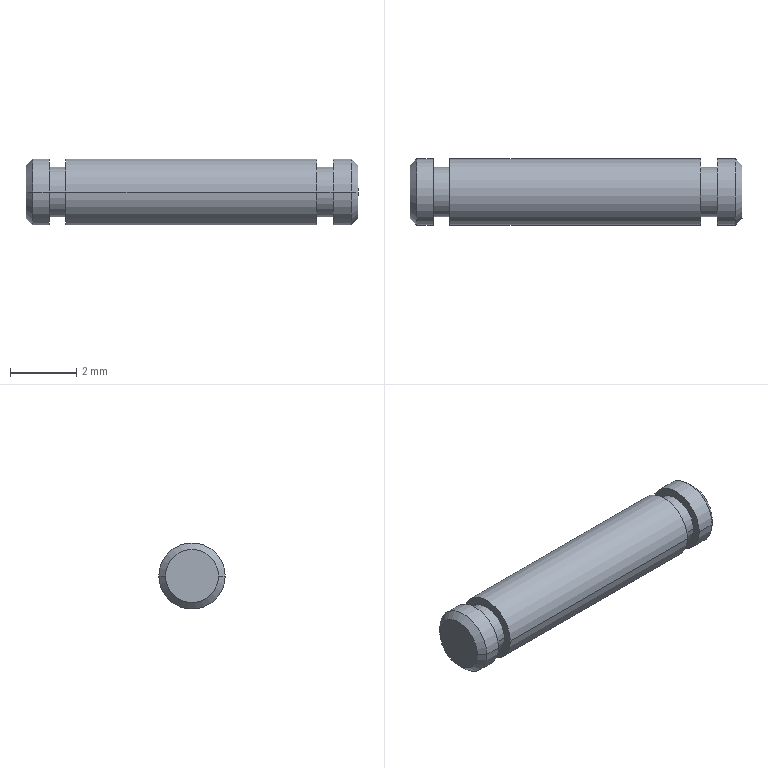Part | NX | 1 solid | 20 faces | box 10 x 2 x 2 mm | volume 29.807 mm3 | cylinder 10 | plane 6 | cone 4 | commonest cylinder face diameters 2 x6 1.5 x4
STEP:
#1=CARTESIAN_POINT('',(-1.16,-50.479,1.703));
#2=VERTEX_POINT('',#1);
#3=CARTESIAN_POINT('',(-1.16,-52.479,1.703));
#4=VERTEX_POINT('',#3);
#5=CARTESIAN_POINT('',(-1.16,-51.479,1.703));
#6=DIRECTION('',(-1.,0.,0.));
#7=DIRECTION('',(0.,-1.,0.));
#8=AXIS2_PLACEMENT_3D('',#5,#6,#7);
#9=CIRCLE('',#8,1.);
#10=EDGE_CURVE('',#2,#4,#9,.T.);
#11=ORIENTED_EDGE('',*,*,#10,.T.);
#12=CARTESIAN_POINT('',(-1.71,-52.479,1.703));
#13=VERTEX_POINT('',#12);
#14=CARTESIAN_POINT('',(-10.96,-52.479,1.703));
#15=DIRECTION('',(-1.,0.,0.));
#16=VECTOR('',#15,1000.);
#17=LINE('',#14,#16);
#18=EDGE_CURVE('',#13,#4,#17,.F.);
#19=ORIENTED_EDGE('',*,*,#18,.F.);
#20=CARTESIAN_POINT('',(-1.71,-50.479,1.703));
#21=VERTEX_POINT('',#20);
#22=CARTESIAN_POINT('',(-1.71,-51.479,1.703));
#23=DIRECTION('',(-1.,0.,0.));
#24=DIRECTION('',(0.,-1.,0.));
#25=AXIS2_PLACEMENT_3D('',#22,#23,#24);
#26=CIRCLE('',#25,1.);
#27=EDGE_CURVE('',#21,#13,#26,.T.);
#28=ORIENTED_EDGE('',*,*,#27,.F.);
#29=CARTESIAN_POINT('',(-10.96,-50.479,1.703));
#30=DIRECTION('',(-1.,0.,0.));
#31=VECTOR('',#30,1000.);
#32=LINE('',#29,#31);
#33=EDGE_CURVE('',#21,#2,#32,.F.);
#34=ORIENTED_EDGE('',*,*,#33,.T.);
#35=EDGE_LOOP('',(#11,#19,#28,#34));
#36=FACE_BOUND('',#35,.T.);
#37=CARTESIAN_POINT('',(-10.96,-51.479,1.703));
#38=DIRECTION('',(-1.,0.,0.));
#39=DIRECTION('',(0.,-1.,0.));
#40=AXIS2_PLACEMENT_3D('',#37,#38,#39);
#41=CYLINDRICAL_SURFACE('',#40,1.);
#42=ADVANCED_FACE('',(#36),#41,.T.);
#43=ORIENTED_EDGE('',*,*,#27,.T.);
#44=CARTESIAN_POINT('',(-1.71,-51.479,1.703));
#45=DIRECTION('',(-1.,0.,0.));
#46=DIRECTION('',(0.,-1.,0.));
#47=AXIS2_PLACEMENT_3D('',#44,#45,#46);
#48=CIRCLE('',#47,1.);
#49=EDGE_CURVE('',#13,#21,#48,.T.);
#50=ORIENTED_EDGE('',*,*,#49,.T.);
#51=EDGE_LOOP('',(#43,#50));
#52=FACE_BOUND('',#51,.T.);
#53=CARTESIAN_POINT('',(-1.71,-50.729,1.703));
#54=VERTEX_POINT('',#53);
#55=CARTESIAN_POINT('',(-1.71,-52.229,1.703));
#56=VERTEX_POINT('',#55);
#57=CARTESIAN_POINT('',(-1.71,-51.479,1.703));
#58=DIRECTION('',(-1.,0.,0.));
#59=DIRECTION('',(0.,-1.,0.));
#60=AXIS2_PLACEMENT_3D('',#57,#58,#59);
#61=CIRCLE('',#60,0.75);
#62=EDGE_CURVE('',#54,#56,#61,.T.);
#63=ORIENTED_EDGE('',*,*,#62,.F.);
#64=CARTESIAN_POINT('',(-1.71,-51.479,1.703));
#65=DIRECTION('',(-1.,0.,0.));
#66=DIRECTION('',(0.,-1.,0.));
#67=AXIS2_PLACEMENT_3D('',#64,#65,#66);
#68=CIRCLE('',#67,0.75);
#69=EDGE_CURVE('',#56,#54,#68,.T.);
#70=ORIENTED_EDGE('',*,*,#69,.F.);
#71=EDGE_LOOP('',(#63,#70));
#72=FACE_BOUND('',#71,.T.);
#73=CARTESIAN_POINT('',(-1.71,-50.265,1.703));
#74=DIRECTION('',(-1.,0.,0.));
#75=DIRECTION('',(0.,1.,0.));
#76=AXIS2_PLACEMENT_3D('',#73,#74,#75);
#77=PLANE('',#76);
#78=ADVANCED_FACE('',(#52,#72),#77,.T.);
#79=CARTESIAN_POINT('',(-2.21,-50.729,1.703));
#80=VERTEX_POINT('',#79);
#81=CARTESIAN_POINT('',(-2.21,-52.229,1.703));
#82=VERTEX_POINT('',#81);
#83=CARTESIAN_POINT('',(-2.21,-51.479,1.703));
#84=DIRECTION('',(-1.,0.,0.));
#85=DIRECTION('',(0.,-1.,0.));
#86=AXIS2_PLACEMENT_3D('',#83,#84,#85);
#87=CIRCLE('',#86,0.75);
#88=EDGE_CURVE('',#80,#82,#87,.T.);
#89=ORIENTED_EDGE('',*,*,#88,.F.);
#90=CARTESIAN_POINT('',(-3.61,-50.729,1.703));
#91=DIRECTION('',(-1.,0.,0.));
#92=VECTOR('',#91,1000.);
#93=LINE('',#90,#92);
#94=EDGE_CURVE('',#80,#54,#93,.F.);
#95=ORIENTED_EDGE('',*,*,#94,.T.);
#96=ORIENTED_EDGE('',*,*,#62,.T.);
#97=CARTESIAN_POINT('',(-3.61,-52.229,1.703));
#98=DIRECTION('',(-1.,0.,0.));
#99=VECTOR('',#98,1000.);
#100=LINE('',#97,#99);
#101=EDGE_CURVE('',#82,#56,#100,.F.);
#102=ORIENTED_EDGE('',*,*,#101,.F.);
#103=EDGE_LOOP('',(#89,#95,#96,#102));
#104=FACE_BOUND('',#103,.T.);
#105=CARTESIAN_POINT('',(-3.61,-51.479,1.703));
#106=DIRECTION('',(-1.,0.,0.));
#107=DIRECTION('',(0.,-1.,0.));
#108=AXIS2_PLACEMENT_3D('',#105,#106,#107);
#109=CYLINDRICAL_SURFACE('',#108,0.75);
#110=ADVANCED_FACE('',(#104),#109,.T.);
#111=CARTESIAN_POINT('',(-10.26,-50.479,1.703));
#112=VERTEX_POINT('',#111);
#113=CARTESIAN_POINT('',(-10.26,-52.479,1.703));
#114=VERTEX_POINT('',#113);
#115=CARTESIAN_POINT('',(-10.26,-51.479,1.703));
#116=DIRECTION('',(-1.,0.,0.));
#117=DIRECTION('',(0.,-1.,0.));
#118=AXIS2_PLACEMENT_3D('',#115,#116,#117);
#119=CIRCLE('',#118,1.);
#120=EDGE_CURVE('',#112,#114,#119,.T.);
#121=ORIENTED_EDGE('',*,*,#120,.T.);
#122=CARTESIAN_POINT('',(-10.76,-52.479,1.703));
#123=VERTEX_POINT('',#122);
#124=CARTESIAN_POINT('',(-10.96,-52.479,1.703));
#125=DIRECTION('',(-1.,0.,0.));
#126=VECTOR('',#125,1000.);
#127=LINE('',#124,#126);
#128=EDGE_CURVE('',#123,#114,#127,.F.);
#129=ORIENTED_EDGE('',*,*,#128,.F.);
#130=CARTESIAN_POINT('',(-10.76,-50.479,1.703));
#131=VERTEX_POINT('',#130);
#132=CARTESIAN_POINT('',(-10.76,-51.479,1.703));
#133=DIRECTION('',(-1.,0.,0.));
#134=DIRECTION('',(0.,-1.,0.));
#135=AXIS2_PLACEMENT_3D('',#132,#133,#134);
#136=CIRCLE('',#135,1.);
#137=EDGE_CURVE('',#131,#123,#136,.T.);
#138=ORIENTED_EDGE('',*,*,#137,.F.);
#139=CARTESIAN_POINT('',(-10.96,-50.479,1.703));
#140=DIRECTION('',(-1.,0.,0.));
#141=VECTOR('',#140,1000.);
#142=LINE('',#139,#141);
#143=EDGE_CURVE('',#131,#112,#142,.F.);
#144=ORIENTED_EDGE('',*,*,#143,.T.);
#145=EDGE_LOOP('',(#121,#129,#138,#144));
#146=FACE_BOUND('',#145,.T.);
#147=CARTESIAN_POINT('',(-10.96,-51.479,1.703));
#148=DIRECTION('',(-1.,0.,0.));
#149=DIRECTION('',(0.,-1.,0.));
#150=AXIS2_PLACEMENT_3D('',#147,#148,#149);
#151=CYLINDRICAL_SURFACE('',#150,1.);
#152=ADVANCED_FACE('',(#146),#151,.T.);
#153=ORIENTED_EDGE('',*,*,#120,.F.);
#154=CARTESIAN_POINT('',(-10.26,-51.479,1.703));
#155=DIRECTION('',(-1.,0.,0.));
#156=DIRECTION('',(0.,-1.,0.));
#157=AXIS2_PLACEMENT_3D('',#154,#155,#156);
#158=CIRCLE('',#157,1.);
#159=EDGE_CURVE('',#114,#112,#158,.T.);
#160=ORIENTED_EDGE('',*,*,#159,.F.);
#161=EDGE_LOOP('',(#153,#160));
#162=FACE_BOUND('',#161,.T.);
#163=CARTESIAN_POINT('',(-10.26,-50.729,1.703));
#164=VERTEX_POINT('',#163);
#165=CARTESIAN_POINT('',(-10.26,-52.229,1.703));
#166=VERTEX_POINT('',#165);
#167=CARTESIAN_POINT('',(-10.26,-51.479,1.703));
#168=DIRECTION('',(-1.,0.,0.));
#169=DIRECTION('',(0.,-1.,0.));
#170=AXIS2_PLACEMENT_3D('',#167,#168,#169);
#171=CIRCLE('',#170,0.75);
#172=EDGE_CURVE('',#164,#166,#171,.T.);
#173=ORIENTED_EDGE('',*,*,#172,.T.);
#174=CARTESIAN_POINT('',(-10.26,-51.479,1.703));
#175=DIRECTION('',(-1.,0.,0.));
#176=DIRECTION('',(0.,-1.,0.));
#177=AXIS2_PLACEMENT_3D('',#174,#175,#176);
#178=CIRCLE('',#177,0.75);
#179=EDGE_CURVE('',#166,#164,#178,.T.);
#180=ORIENTED_EDGE('',*,*,#179,.T.);
#181=EDGE_LOOP('',(#173,#180));
#182=FACE_BOUND('',#181,.T.);
#183=CARTESIAN_POINT('',(-10.26,-50.389,1.703));
#184=DIRECTION('',(-1.,0.,0.));
#185=DIRECTION('',(0.,1.,0.));
#186=AXIS2_PLACEMENT_3D('',#183,#184,#185);
#187=PLANE('',#186);
#188=ADVANCED_FACE('',(#162,#182),#187,.F.);
#189=ORIENTED_EDGE('',*,*,#172,.F.);
#190=CARTESIAN_POINT('',(-9.76,-50.729,1.703));
#191=VERTEX_POINT('',#190);
#192=CARTESIAN_POINT('',(-10.01,-50.729,1.703));
#193=DIRECTION('',(-1.,0.,0.));
#194=VECTOR('',#193,1000.);
#195=LINE('',#192,#194);
#196=EDGE_CURVE('',#164,#191,#195,.F.);
#197=ORIENTED_EDGE('',*,*,#196,.T.);
#198=CARTESIAN_POINT('',(-9.76,-52.229,1.703));
#199=VERTEX_POINT('',#198);
#200=CARTESIAN_POINT('',(-9.76,-51.479,1.703));
#201=DIRECTION('',(-1.,0.,0.));
#202=DIRECTION('',(0.,-1.,0.));
#203=AXIS2_PLACEMENT_3D('',#200,#201,#202);
#204=CIRCLE('',#203,0.75);
#205=EDGE_CURVE('',#191,#199,#204,.T.);
#206=ORIENTED_EDGE('',*,*,#205,.T.);
#207=CARTESIAN_POINT('',(-10.01,-52.229,1.703));
#208=DIRECTION('',(-1.,0.,0.));
#209=VECTOR('',#208,1000.);
#210=LINE('',#207,#209);
#211=EDGE_CURVE('',#166,#199,#210,.F.);
#212=ORIENTED_EDGE('',*,*,#211,.F.);
#213=EDGE_LOOP('',(#189,#197,#206,#212));
#214=FACE_BOUND('',#213,.T.);
#215=CARTESIAN_POINT('',(-10.01,-51.479,1.703));
#216=DIRECTION('',(-1.,0.,0.));
#217=DIRECTION('',(0.,-1.,0.));
#218=AXIS2_PLACEMENT_3D('',#215,#216,#217);
#219=CYLINDRICAL_SURFACE('',#218,0.75);
#220=ADVANCED_FACE('',(#214),#219,.T.);
#221=CARTESIAN_POINT('',(-9.76,-50.479,1.703));
#222=VERTEX_POINT('',#221);
#223=CARTESIAN_POINT('',(-9.76,-52.479,1.703));
#224=VERTEX_POINT('',#223);
#225=CARTESIAN_POINT('',(-9.76,-51.479,1.703));
#226=DIRECTION('',(-1.,0.,0.));
#227=DIRECTION('',(0.,-1.,0.));
#228=AXIS2_PLACEMENT_3D('',#225,#226,#227);
#229=CIRCLE('',#228,1.);
#230=EDGE_CURVE('',#222,#224,#229,.T.);
#231=ORIENTED_EDGE('',*,*,#230,.T.);
#232=CARTESIAN_POINT('',(-9.76,-51.479,1.703));
#233=DIRECTION('',(-1.,0.,0.));
#234=DIRECTION('',(0.,-1.,0.));
#235=AXIS2_PLACEMENT_3D('',#232,#233,#234);
#236=CIRCLE('',#235,1.);
#237=EDGE_CURVE('',#224,#222,#236,.T.);
#238=ORIENTED_EDGE('',*,*,#237,.T.);
#239=EDGE_LOOP('',(#231,#238));
#240=FACE_BOUND('',#239,.T.);
#241=ORIENTED_EDGE('',*,*,#205,.F.);
#242=CARTESIAN_POINT('',(-9.76,-51.479,1.703));
#243=DIRECTION('',(-1.,0.,0.));
#244=DIRECTION('',(0.,-1.,0.));
#245=AXIS2_PLACEMENT_3D('',#242,#243,#244);
#246=CIRCLE('',#245,0.75);
#247=EDGE_CURVE('',#199,#191,#246,.T.);
#248=ORIENTED_EDGE('',*,*,#247,.F.);
#249=EDGE_LOOP('',(#241,#248));
#250=FACE_BOUND('',#249,.T.);
#251=CARTESIAN_POINT('',(-9.76,-50.329,1.703));
#252=DIRECTION('',(1.,0.,0.));
#253=DIRECTION('',(0.,1.,0.));
#254=AXIS2_PLACEMENT_3D('',#251,#252,#253);
#255=PLANE('',#254);
#256=ADVANCED_FACE('',(#240,#250),#255,.F.);
#257=CARTESIAN_POINT('',(-2.21,-50.479,1.703));
#258=VERTEX_POINT('',#257);
#259=CARTESIAN_POINT('',(-2.21,-52.479,1.703));
#260=VERTEX_POINT('',#259);
#261=CARTESIAN_POINT('',(-2.21,-51.479,1.703));
#262=DIRECTION('',(-1.,0.,0.));
#263=DIRECTION('',(0.,-1.,0.));
#264=AXIS2_PLACEMENT_3D('',#261,#262,#263);
#265=CIRCLE('',#264,1.);
#266=EDGE_CURVE('',#258,#260,#265,.T.);
#267=ORIENTED_EDGE('',*,*,#266,.T.);
#268=CARTESIAN_POINT('',(-10.96,-52.479,1.703));
#269=DIRECTION('',(-1.,0.,0.));
#270=VECTOR('',#269,1000.);
#271=LINE('',#268,#270);
#272=EDGE_CURVE('',#224,#260,#271,.F.);
#273=ORIENTED_EDGE('',*,*,#272,.F.);
#274=ORIENTED_EDGE('',*,*,#230,.F.);
#275=CARTESIAN_POINT('',(-10.96,-50.479,1.703));
#276=DIRECTION('',(-1.,0.,0.));
#277=VECTOR('',#276,1000.);
#278=LINE('',#275,#277);
#279=EDGE_CURVE('',#222,#258,#278,.F.);
#280=ORIENTED_EDGE('',*,*,#279,.T.);
#281=EDGE_LOOP('',(#267,#273,#274,#280));
#282=FACE_BOUND('',#281,.T.);
#283=CARTESIAN_POINT('',(-10.96,-51.479,1.703));
#284=DIRECTION('',(-1.,0.,0.));
#285=DIRECTION('',(0.,-1.,0.));
#286=AXIS2_PLACEMENT_3D('',#283,#284,#285);
#287=CYLINDRICAL_SURFACE('',#286,1.);
#288=ADVANCED_FACE('',(#282),#287,.T.);
#289=ORIENTED_EDGE('',*,*,#266,.F.);
#290=CARTESIAN_POINT('',(-2.21,-51.479,1.703));
#291=DIRECTION('',(-1.,0.,0.));
#292=DIRECTION('',(0.,-1.,0.));
#293=AXIS2_PLACEMENT_3D('',#290,#291,#292);
#294=CIRCLE('',#293,1.);
#295=EDGE_CURVE('',#260,#258,#294,.T.);
#296=ORIENTED_EDGE('',*,*,#295,.F.);
#297=EDGE_LOOP('',(#289,#296));
#298=FACE_BOUND('',#297,.T.);
#299=ORIENTED_EDGE('',*,*,#88,.T.);
#300=CARTESIAN_POINT('',(-2.21,-51.479,1.703));
#301=DIRECTION('',(-1.,0.,0.));
#302=DIRECTION('',(0.,-1.,0.));
#303=AXIS2_PLACEMENT_3D('',#300,#301,#302);
#304=CIRCLE('',#303,0.75);
#305=EDGE_CURVE('',#82,#80,#304,.T.);
#306=ORIENTED_EDGE('',*,*,#305,.T.);
#307=EDGE_LOOP('',(#299,#306));
#308=FACE_BOUND('',#307,.T.);
#309=CARTESIAN_POINT('',(-2.21,-50.325,1.703));
#310=DIRECTION('',(1.,0.,0.));
#311=DIRECTION('',(0.,1.,0.));
#312=AXIS2_PLACEMENT_3D('',#309,#310,#311);
#313=PLANE('',#312);
#314=ADVANCED_FACE('',(#298,#308),#313,.T.);
#315=ORIENTED_EDGE('',*,*,#101,.T.);
#316=ORIENTED_EDGE('',*,*,#69,.T.);
#317=ORIENTED_EDGE('',*,*,#94,.F.);
#318=ORIENTED_EDGE('',*,*,#305,.F.);
#319=EDGE_LOOP('',(#315,#316,#317,#318));
#320=FACE_BOUND('',#319,.T.);
#321=CARTESIAN_POINT('',(-3.61,-51.479,1.703));
#322=DIRECTION('',(-1.,0.,0.));
#323=DIRECTION('',(0.,-1.,0.));
#324=AXIS2_PLACEMENT_3D('',#321,#322,#323);
#325=CYLINDRICAL_SURFACE('',#324,0.75);
#326=ADVANCED_FACE('',(#320),#325,.T.);
#327=ORIENTED_EDGE('',*,*,#128,.T.);
#328=ORIENTED_EDGE('',*,*,#159,.T.);
#329=ORIENTED_EDGE('',*,*,#143,.F.);
#330=CARTESIAN_POINT('',(-10.76,-51.479,1.703));
#331=DIRECTION('',(-1.,0.,0.));
#332=DIRECTION('',(0.,-1.,0.));
#333=AXIS2_PLACEMENT_3D('',#330,#331,#332);
#334=CIRCLE('',#333,1.);
#335=EDGE_CURVE('',#123,#131,#334,.T.);
#336=ORIENTED_EDGE('',*,*,#335,.F.);
#337=EDGE_LOOP('',(#327,#328,#329,#336));
#338=FACE_BOUND('',#337,.T.);
#339=CARTESIAN_POINT('',(-10.96,-51.479,1.703));
#340=DIRECTION('',(-1.,0.,0.));
#341=DIRECTION('',(0.,-1.,0.));
#342=AXIS2_PLACEMENT_3D('',#339,#340,#341);
#343=CYLINDRICAL_SURFACE('',#342,1.);
#344=ADVANCED_FACE('',(#338),#343,.T.);
#345=ORIENTED_EDGE('',*,*,#211,.T.);
#346=ORIENTED_EDGE('',*,*,#247,.T.);
#347=ORIENTED_EDGE('',*,*,#196,.F.);
#348=ORIENTED_EDGE('',*,*,#179,.F.);
#349=EDGE_LOOP('',(#345,#346,#347,#348));
#350=FACE_BOUND('',#349,.T.);
#351=CARTESIAN_POINT('',(-10.01,-51.479,1.703));
#352=DIRECTION('',(-1.,0.,0.));
#353=DIRECTION('',(0.,-1.,0.));
#354=AXIS2_PLACEMENT_3D('',#351,#352,#353);
#355=CYLINDRICAL_SURFACE('',#354,0.75);
#356=ADVANCED_FACE('',(#350),#355,.T.);
#357=ORIENTED_EDGE('',*,*,#18,.T.);
#358=CARTESIAN_POINT('',(-1.16,-51.479,1.703));
#359=DIRECTION('',(-1.,0.,0.));
#360=DIRECTION('',(0.,-1.,0.));
#361=AXIS2_PLACEMENT_3D('',#358,#359,#360);
#362=CIRCLE('',#361,1.);
#363=EDGE_CURVE('',#4,#2,#362,.T.);
#364=ORIENTED_EDGE('',*,*,#363,.T.);
#365=ORIENTED_EDGE('',*,*,#33,.F.);
#366=ORIENTED_EDGE('',*,*,#49,.F.);
#367=EDGE_LOOP('',(#357,#364,#365,#366));
#368=FACE_BOUND('',#367,.T.);
#369=CARTESIAN_POINT('',(-10.96,-51.479,1.703));
#370=DIRECTION('',(-1.,0.,0.));
#371=DIRECTION('',(0.,-1.,0.));
#372=AXIS2_PLACEMENT_3D('',#369,#370,#371);
#373=CYLINDRICAL_SURFACE('',#372,1.);
#374=ADVANCED_FACE('',(#368),#373,.T.);
#375=ORIENTED_EDGE('',*,*,#272,.T.);
#376=ORIENTED_EDGE('',*,*,#295,.T.);
#377=ORIENTED_EDGE('',*,*,#279,.F.);
#378=ORIENTED_EDGE('',*,*,#237,.F.);
#379=EDGE_LOOP('',(#375,#376,#377,#378));
#380=FACE_BOUND('',#379,.T.);
#381=CARTESIAN_POINT('',(-10.96,-51.479,1.703));
#382=DIRECTION('',(-1.,0.,0.));
#383=DIRECTION('',(0.,-1.,0.));
#384=AXIS2_PLACEMENT_3D('',#381,#382,#383);
#385=CYLINDRICAL_SURFACE('',#384,1.);
#386=ADVANCED_FACE('',(#380),#385,.T.);
#387=CARTESIAN_POINT('',(-0.9603,-50.679,1.703));
#388=VERTEX_POINT('',#387);
#389=CARTESIAN_POINT('',(-0.9603,-52.279,1.703));
#390=VERTEX_POINT('',#389);
#391=CARTESIAN_POINT('',(-0.9603,-51.479,1.703));
#392=DIRECTION('',(-1.,0.,0.));
#393=DIRECTION('',(0.,-1.,0.));
#394=AXIS2_PLACEMENT_3D('',#391,#392,#393);
#395=CIRCLE('',#394,0.8);
#396=EDGE_CURVE('',#388,#390,#395,.T.);
#397=ORIENTED_EDGE('',*,*,#396,.F.);
#398=CARTESIAN_POINT('',(-0.9603,-51.479,1.703));
#399=DIRECTION('',(-1.,0.,0.));
#400=DIRECTION('',(0.,-1.,0.));
#401=AXIS2_PLACEMENT_3D('',#398,#399,#400);
#402=CIRCLE('',#401,0.8);
#403=EDGE_CURVE('',#390,#388,#402,.T.);
#404=ORIENTED_EDGE('',*,*,#403,.F.);
#405=EDGE_LOOP('',(#397,#404));
#406=FACE_BOUND('',#405,.T.);
#407=CARTESIAN_POINT('',(-0.9603,-53.706,-1.894));
#408=DIRECTION('',(-1.,0.,0.));
#409=DIRECTION('',(0.,1.,0.));
#410=AXIS2_PLACEMENT_3D('',#407,#408,#409);
#411=PLANE('',#410);
#412=ADVANCED_FACE('',(#406),#411,.F.);
#413=ORIENTED_EDGE('',*,*,#396,.T.);
#414=CARTESIAN_POINT('',(-0.9603,-52.279,1.703));
#415=DIRECTION('',(-0.7071,-0.7071,0.));
#416=VECTOR('',#415,1000.);
#417=LINE('',#414,#416);
#418=EDGE_CURVE('',#4,#390,#417,.F.);
#419=ORIENTED_EDGE('',*,*,#418,.F.);
#420=ORIENTED_EDGE('',*,*,#10,.F.);
#421=CARTESIAN_POINT('',(-0.9603,-50.679,1.703));
#422=DIRECTION('',(-0.7071,0.7071,0.));
#423=VECTOR('',#422,1000.);
#424=LINE('',#421,#423);
#425=EDGE_CURVE('',#2,#388,#424,.F.);
#426=ORIENTED_EDGE('',*,*,#425,.T.);
#427=EDGE_LOOP('',(#413,#419,#420,#426));
#428=FACE_BOUND('',#427,.T.);
#429=CARTESIAN_POINT('',(-0.9603,-51.479,1.703));
#430=DIRECTION('',(-1.,0.,0.));
#431=DIRECTION('',(0.,-1.,0.));
#432=AXIS2_PLACEMENT_3D('',#429,#430,#431);
#433=CONICAL_SURFACE('',#432,0.8,0.7854);
#434=ADVANCED_FACE('',(#428),#433,.T.);
#435=ORIENTED_EDGE('',*,*,#418,.T.);
#436=ORIENTED_EDGE('',*,*,#403,.T.);
#437=ORIENTED_EDGE('',*,*,#425,.F.);
#438=ORIENTED_EDGE('',*,*,#363,.F.);
#439=EDGE_LOOP('',(#435,#436,#437,#438));
#440=FACE_BOUND('',#439,.T.);
#441=CARTESIAN_POINT('',(-0.9603,-51.479,1.703));
#442=DIRECTION('',(-1.,0.,0.));
#443=DIRECTION('',(0.,-1.,0.));
#444=AXIS2_PLACEMENT_3D('',#441,#442,#443);
#445=CONICAL_SURFACE('',#444,0.8,0.7854);
#446=ADVANCED_FACE('',(#440),#445,.T.);
#447=CARTESIAN_POINT('',(-10.96,-50.679,1.703));
#448=VERTEX_POINT('',#447);
#449=CARTESIAN_POINT('',(-10.96,-52.279,1.703));
#450=VERTEX_POINT('',#449);
#451=CARTESIAN_POINT('',(-10.96,-51.479,1.703));
#452=DIRECTION('',(-1.,0.,0.));
#453=DIRECTION('',(0.,-1.,0.));
#454=AXIS2_PLACEMENT_3D('',#451,#452,#453);
#455=CIRCLE('',#454,0.8);
#456=EDGE_CURVE('',#448,#450,#455,.T.);
#457=ORIENTED_EDGE('',*,*,#456,.T.);
#458=CARTESIAN_POINT('',(-10.96,-51.479,1.703));
#459=DIRECTION('',(-1.,0.,0.));
#460=DIRECTION('',(0.,-1.,0.));
#461=AXIS2_PLACEMENT_3D('',#458,#459,#460);
#462=CIRCLE('',#461,0.8);
#463=EDGE_CURVE('',#450,#448,#462,.T.);
#464=ORIENTED_EDGE('',*,*,#463,.T.);
#465=EDGE_LOOP('',(#457,#464));
#466=FACE_BOUND('',#465,.T.);
#467=CARTESIAN_POINT('',(-10.96,-53.706,-1.894));
#468=DIRECTION('',(-1.,0.,0.));
#469=DIRECTION('',(0.,1.,0.));
#470=AXIS2_PLACEMENT_3D('',#467,#468,#469);
#471=PLANE('',#470);
#472=ADVANCED_FACE('',(#466),#471,.T.);
#473=ORIENTED_EDGE('',*,*,#456,.F.);
#474=CARTESIAN_POINT('',(-10.96,-50.679,1.703));
#475=DIRECTION('',(0.7071,0.7071,0.));
#476=VECTOR('',#475,1000.);
#477=LINE('',#474,#476);
#478=EDGE_CURVE('',#448,#131,#477,.T.);
#479=ORIENTED_EDGE('',*,*,#478,.T.);
#480=ORIENTED_EDGE('',*,*,#137,.T.);
#481=CARTESIAN_POINT('',(-10.96,-52.279,1.703));
#482=DIRECTION('',(0.7071,-0.7071,0.));
#483=VECTOR('',#482,1000.);
#484=LINE('',#481,#483);
#485=EDGE_CURVE('',#450,#123,#484,.T.);
#486=ORIENTED_EDGE('',*,*,#485,.F.);
#487=EDGE_LOOP('',(#473,#479,#480,#486));
#488=FACE_BOUND('',#487,.T.);
#489=CARTESIAN_POINT('',(-10.96,-51.479,1.703));
#490=DIRECTION('',(1.,0.,0.));
#491=DIRECTION('',(0.,1.,0.));
#492=AXIS2_PLACEMENT_3D('',#489,#490,#491);
#493=CONICAL_SURFACE('',#492,0.8,0.7854);
#494=ADVANCED_FACE('',(#488),#493,.T.);
#495=ORIENTED_EDGE('',*,*,#478,.F.);
#496=ORIENTED_EDGE('',*,*,#463,.F.);
#497=ORIENTED_EDGE('',*,*,#485,.T.);
#498=ORIENTED_EDGE('',*,*,#335,.T.);
#499=EDGE_LOOP('',(#495,#496,#497,#498));
#500=FACE_BOUND('',#499,.T.);
#501=CARTESIAN_POINT('',(-10.96,-51.479,1.703));
#502=DIRECTION('',(1.,0.,0.));
#503=DIRECTION('',(0.,1.,0.));
#504=AXIS2_PLACEMENT_3D('',#501,#502,#503);
#505=CONICAL_SURFACE('',#504,0.8,0.7854);
#506=ADVANCED_FACE('',(#500),#505,.T.);
#507=CLOSED_SHELL('',(#42,#78,#110,#152,#188,#220,#256,#288,#314,#326,#344,#356,#374,#386,#412,#434,#446,#472,#494,#506));
#508=MANIFOLD_SOLID_BREP('',#507);
#509=(LENGTH_UNIT()NAMED_UNIT(*)SI_UNIT(.MILLI.,.METRE.));
#510=UNCERTAINTY_MEASURE_WITH_UNIT(LENGTH_MEASURE(0.00001),#509,'','');
#511=(NAMED_UNIT(*)PLANE_ANGLE_UNIT()SI_UNIT($,.RADIAN.));
#512=(NAMED_UNIT(*)SI_UNIT($,.STERADIAN.)SOLID_ANGLE_UNIT());
#513=(GEOMETRIC_REPRESENTATION_CONTEXT(3)GLOBAL_UNCERTAINTY_ASSIGNED_CONTEXT((#510))GLOBAL_UNIT_ASSIGNED_CONTEXT((#509,#511,#512))REPRESENTATION_CONTEXT('',''));
#514=ADVANCED_BREP_SHAPE_REPRESENTATION('',(#508),#513);